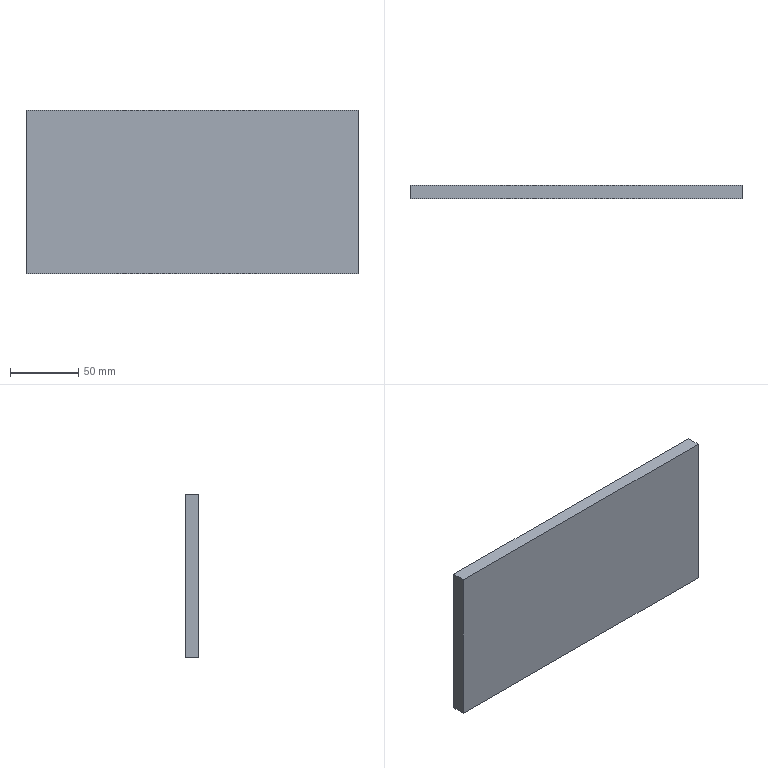Part | STEP file | 1 solid | 6 faces | box 243.554 x 10 x 120 mm | volume 292264 mm3 | plane 6
STEP:
#1=CARTESIAN_POINT('',(0.,0.,0.));
#2=DIRECTION('',(0.,0.,1.));
#3=DIRECTION('',(1.,0.,0.));
#4=AXIS2_PLACEMENT_3D('',#1,#2,#3);
#5=CARTESIAN_POINT('',(-600.,430.,-60.));
#6=VERTEX_POINT('',#5);
#7=CARTESIAN_POINT('',(-600.,430.,60.));
#8=VERTEX_POINT('',#7);
#9=CARTESIAN_POINT('',(-600.,430.,-60.));
#10=DIRECTION('',(0.,0.,1.));
#11=VECTOR('',#10,1.);
#12=LINE('',#9,#11);
#13=CARTESIAN_POINT('',(-600.,440.,-60.));
#14=DIRECTION('',(1.,0.,0.));
#15=DIRECTION('',(0.,1.,0.));
#16=AXIS2_PLACEMENT_3D('',#13,#14,#15);
#17=PLANE('',#16);
#18=CARTESIAN_POINT('',(-10.,0.));
#19=DIRECTION('',(0.,1.));
#20=VECTOR('',#19,1.);
#21=LINE('',#18,#20);
#22=(GEOMETRIC_REPRESENTATION_CONTEXT(2)PARAMETRIC_REPRESENTATION_CONTEXT()REPRESENTATION_CONTEXT('',''));
#23=DEFINITIONAL_REPRESENTATION('',(#21),#22);
#24=PCURVE('',#17,#23);
#25=CARTESIAN_POINT('',(0.,430.,0.));
#26=DIRECTION('',(0.,1.,0.));
#27=DIRECTION('',(0.,0.,1.));
#28=AXIS2_PLACEMENT_3D('',#25,#26,#27);
#29=PLANE('',#28);
#30=CARTESIAN_POINT('',(-60.,-600.));
#31=DIRECTION('',(1.,0.));
#32=VECTOR('',#31,1.);
#33=LINE('',#30,#32);
#34=(GEOMETRIC_REPRESENTATION_CONTEXT(2)PARAMETRIC_REPRESENTATION_CONTEXT()REPRESENTATION_CONTEXT('',''));
#35=DEFINITIONAL_REPRESENTATION('',(#33),#34);
#36=PCURVE('',#29,#35);
#37=SURFACE_CURVE('',#12,(#24,#36),.PCURVE_S1.);
#38=EDGE_CURVE('',#6,#8,#37,.T.);
#39=ORIENTED_EDGE('',*,*,#38,.T.);
#40=CARTESIAN_POINT('',(-600.,440.,60.));
#41=VERTEX_POINT('',#40);
#42=CARTESIAN_POINT('',(-600.,440.,60.));
#43=DIRECTION('',(0.,-1.,0.));
#44=VECTOR('',#43,1.);
#45=LINE('',#42,#44);
#46=CARTESIAN_POINT('',(0.,120.));
#47=DIRECTION('',(-1.,0.));
#48=VECTOR('',#47,1.);
#49=LINE('',#46,#48);
#50=(GEOMETRIC_REPRESENTATION_CONTEXT(2)PARAMETRIC_REPRESENTATION_CONTEXT()REPRESENTATION_CONTEXT('',''));
#51=DEFINITIONAL_REPRESENTATION('',(#49),#50);
#52=PCURVE('',#17,#51);
#53=CARTESIAN_POINT('',(-600.,440.,60.));
#54=DIRECTION('',(0.,0.,-1.));
#55=DIRECTION('',(-1.,0.,0.));
#56=AXIS2_PLACEMENT_3D('',#53,#54,#55);
#57=PLANE('',#56);
#58=CARTESIAN_POINT('',(0.,0.));
#59=DIRECTION('',(0.,-1.));
#60=VECTOR('',#59,1.);
#61=LINE('',#58,#60);
#62=(GEOMETRIC_REPRESENTATION_CONTEXT(2)PARAMETRIC_REPRESENTATION_CONTEXT()REPRESENTATION_CONTEXT('',''));
#63=DEFINITIONAL_REPRESENTATION('',(#61),#62);
#64=PCURVE('',#57,#63);
#65=SURFACE_CURVE('',#45,(#52,#64),.PCURVE_S1.);
#66=EDGE_CURVE('',#41,#8,#65,.T.);
#67=ORIENTED_EDGE('',*,*,#66,.F.);
#68=CARTESIAN_POINT('',(-600.,440.,-60.));
#69=VERTEX_POINT('',#68);
#70=CARTESIAN_POINT('',(-600.,440.,-60.));
#71=DIRECTION('',(0.,0.,1.));
#72=VECTOR('',#71,1.);
#73=LINE('',#70,#72);
#74=CARTESIAN_POINT('',(0.,0.));
#75=DIRECTION('',(0.,1.));
#76=VECTOR('',#75,1.);
#77=LINE('',#74,#76);
#78=(GEOMETRIC_REPRESENTATION_CONTEXT(2)PARAMETRIC_REPRESENTATION_CONTEXT()REPRESENTATION_CONTEXT('',''));
#79=DEFINITIONAL_REPRESENTATION('',(#77),#78);
#80=PCURVE('',#17,#79);
#81=CARTESIAN_POINT('',(0.,440.,0.));
#82=DIRECTION('',(0.,1.,0.));
#83=DIRECTION('',(0.,0.,1.));
#84=AXIS2_PLACEMENT_3D('',#81,#82,#83);
#85=PLANE('',#84);
#86=CARTESIAN_POINT('',(-60.,-600.));
#87=DIRECTION('',(1.,0.));
#88=VECTOR('',#87,1.);
#89=LINE('',#86,#88);
#90=(GEOMETRIC_REPRESENTATION_CONTEXT(2)PARAMETRIC_REPRESENTATION_CONTEXT()REPRESENTATION_CONTEXT('',''));
#91=DEFINITIONAL_REPRESENTATION('',(#89),#90);
#92=PCURVE('',#85,#91);
#93=SURFACE_CURVE('',#73,(#80,#92),.PCURVE_S1.);
#94=EDGE_CURVE('',#69,#41,#93,.T.);
#95=ORIENTED_EDGE('',*,*,#94,.F.);
#96=CARTESIAN_POINT('',(-600.,440.,-60.));
#97=DIRECTION('',(0.,-1.,0.));
#98=VECTOR('',#97,1.);
#99=LINE('',#96,#98);
#100=CARTESIAN_POINT('',(0.,0.));
#101=DIRECTION('',(-1.,0.));
#102=VECTOR('',#101,1.);
#103=LINE('',#100,#102);
#104=(GEOMETRIC_REPRESENTATION_CONTEXT(2)PARAMETRIC_REPRESENTATION_CONTEXT()REPRESENTATION_CONTEXT('',''));
#105=DEFINITIONAL_REPRESENTATION('',(#103),#104);
#106=PCURVE('',#17,#105);
#107=CARTESIAN_POINT('',(-600.,440.,-60.));
#108=DIRECTION('',(0.,0.,1.));
#109=DIRECTION('',(1.,0.,0.));
#110=AXIS2_PLACEMENT_3D('',#107,#108,#109);
#111=PLANE('',#110);
#112=CARTESIAN_POINT('',(0.,0.));
#113=DIRECTION('',(0.,-1.));
#114=VECTOR('',#113,1.);
#115=LINE('',#112,#114);
#116=(GEOMETRIC_REPRESENTATION_CONTEXT(2)PARAMETRIC_REPRESENTATION_CONTEXT()REPRESENTATION_CONTEXT('',''));
#117=DEFINITIONAL_REPRESENTATION('',(#115),#116);
#118=PCURVE('',#111,#117);
#119=SURFACE_CURVE('',#99,(#106,#118),.PCURVE_S1.);
#120=EDGE_CURVE('',#69,#6,#119,.T.);
#121=ORIENTED_EDGE('',*,*,#120,.T.);
#122=EDGE_LOOP('',(#39,#67,#95,#121));
#123=FACE_BOUND('',#122,.T.);
#124=ADVANCED_FACE('',(#123),#17,.F.);
#125=CARTESIAN_POINT('',(-356.446,430.,60.));
#126=VERTEX_POINT('',#125);
#127=CARTESIAN_POINT('',(-600.,430.,60.));
#128=DIRECTION('',(1.,0.,0.));
#129=VECTOR('',#128,1.);
#130=LINE('',#127,#129);
#131=CARTESIAN_POINT('',(0.,-10.));
#132=DIRECTION('',(-1.,0.));
#133=VECTOR('',#132,1.);
#134=LINE('',#131,#133);
#135=(GEOMETRIC_REPRESENTATION_CONTEXT(2)PARAMETRIC_REPRESENTATION_CONTEXT()REPRESENTATION_CONTEXT('',''));
#136=DEFINITIONAL_REPRESENTATION('',(#134),#135);
#137=PCURVE('',#57,#136);
#138=CARTESIAN_POINT('',(60.,-600.));
#139=DIRECTION('',(0.,1.));
#140=VECTOR('',#139,1.);
#141=LINE('',#138,#140);
#142=(GEOMETRIC_REPRESENTATION_CONTEXT(2)PARAMETRIC_REPRESENTATION_CONTEXT()REPRESENTATION_CONTEXT('',''));
#143=DEFINITIONAL_REPRESENTATION('',(#141),#142);
#144=PCURVE('',#29,#143);
#145=SURFACE_CURVE('',#130,(#137,#144),.PCURVE_S1.);
#146=EDGE_CURVE('',#8,#126,#145,.T.);
#147=ORIENTED_EDGE('',*,*,#146,.T.);
#148=CARTESIAN_POINT('',(-356.446,440.,60.));
#149=VERTEX_POINT('',#148);
#150=CARTESIAN_POINT('',(-356.446,440.,60.));
#151=DIRECTION('',(0.,-1.,0.));
#152=VECTOR('',#151,1.);
#153=LINE('',#150,#152);
#154=CARTESIAN_POINT('',(-243.554,0.));
#155=DIRECTION('',(0.,-1.));
#156=VECTOR('',#155,1.);
#157=LINE('',#154,#156);
#158=(GEOMETRIC_REPRESENTATION_CONTEXT(2)PARAMETRIC_REPRESENTATION_CONTEXT()REPRESENTATION_CONTEXT('',''));
#159=DEFINITIONAL_REPRESENTATION('',(#157),#158);
#160=PCURVE('',#57,#159);
#161=CARTESIAN_POINT('',(-356.446,440.,-60.));
#162=DIRECTION('',(-1.,0.,0.));
#163=DIRECTION('',(0.,-1.,0.));
#164=AXIS2_PLACEMENT_3D('',#161,#162,#163);
#165=PLANE('',#164);
#166=CARTESIAN_POINT('',(0.,120.));
#167=DIRECTION('',(1.,0.));
#168=VECTOR('',#167,1.);
#169=LINE('',#166,#168);
#170=(GEOMETRIC_REPRESENTATION_CONTEXT(2)PARAMETRIC_REPRESENTATION_CONTEXT()REPRESENTATION_CONTEXT('',''));
#171=DEFINITIONAL_REPRESENTATION('',(#169),#170);
#172=PCURVE('',#165,#171);
#173=SURFACE_CURVE('',#153,(#160,#172),.PCURVE_S1.);
#174=EDGE_CURVE('',#149,#126,#173,.T.);
#175=ORIENTED_EDGE('',*,*,#174,.F.);
#176=CARTESIAN_POINT('',(-600.,440.,60.));
#177=DIRECTION('',(1.,0.,0.));
#178=VECTOR('',#177,1.);
#179=LINE('',#176,#178);
#180=CARTESIAN_POINT('',(0.,0.));
#181=DIRECTION('',(-1.,0.));
#182=VECTOR('',#181,1.);
#183=LINE('',#180,#182);
#184=(GEOMETRIC_REPRESENTATION_CONTEXT(2)PARAMETRIC_REPRESENTATION_CONTEXT()REPRESENTATION_CONTEXT('',''));
#185=DEFINITIONAL_REPRESENTATION('',(#183),#184);
#186=PCURVE('',#57,#185);
#187=CARTESIAN_POINT('',(60.,-600.));
#188=DIRECTION('',(0.,1.));
#189=VECTOR('',#188,1.);
#190=LINE('',#187,#189);
#191=(GEOMETRIC_REPRESENTATION_CONTEXT(2)PARAMETRIC_REPRESENTATION_CONTEXT()REPRESENTATION_CONTEXT('',''));
#192=DEFINITIONAL_REPRESENTATION('',(#190),#191);
#193=PCURVE('',#85,#192);
#194=SURFACE_CURVE('',#179,(#186,#193),.PCURVE_S1.);
#195=EDGE_CURVE('',#41,#149,#194,.T.);
#196=ORIENTED_EDGE('',*,*,#195,.F.);
#197=ORIENTED_EDGE('',*,*,#66,.T.);
#198=EDGE_LOOP('',(#147,#175,#196,#197));
#199=FACE_BOUND('',#198,.T.);
#200=ADVANCED_FACE('',(#199),#57,.F.);
#201=CARTESIAN_POINT('',(-356.446,430.,-60.));
#202=VERTEX_POINT('',#201);
#203=CARTESIAN_POINT('',(-356.446,430.,-60.));
#204=DIRECTION('',(0.,0.,-1.));
#205=VECTOR('',#204,1.);
#206=LINE('',#203,#205);
#207=CARTESIAN_POINT('',(10.,0.));
#208=DIRECTION('',(0.,-1.));
#209=VECTOR('',#208,1.);
#210=LINE('',#207,#209);
#211=(GEOMETRIC_REPRESENTATION_CONTEXT(2)PARAMETRIC_REPRESENTATION_CONTEXT()REPRESENTATION_CONTEXT('',''));
#212=DEFINITIONAL_REPRESENTATION('',(#210),#211);
#213=PCURVE('',#165,#212);
#214=CARTESIAN_POINT('',(-60.,-356.446));
#215=DIRECTION('',(-1.,0.));
#216=VECTOR('',#215,1.);
#217=LINE('',#214,#216);
#218=(GEOMETRIC_REPRESENTATION_CONTEXT(2)PARAMETRIC_REPRESENTATION_CONTEXT()REPRESENTATION_CONTEXT('',''));
#219=DEFINITIONAL_REPRESENTATION('',(#217),#218);
#220=PCURVE('',#29,#219);
#221=SURFACE_CURVE('',#206,(#213,#220),.PCURVE_S1.);
#222=EDGE_CURVE('',#126,#202,#221,.T.);
#223=ORIENTED_EDGE('',*,*,#222,.T.);
#224=CARTESIAN_POINT('',(-356.446,440.,-60.));
#225=VERTEX_POINT('',#224);
#226=CARTESIAN_POINT('',(-356.446,440.,-60.));
#227=DIRECTION('',(0.,-1.,0.));
#228=VECTOR('',#227,1.);
#229=LINE('',#226,#228);
#230=CARTESIAN_POINT('',(0.,0.));
#231=DIRECTION('',(1.,0.));
#232=VECTOR('',#231,1.);
#233=LINE('',#230,#232);
#234=(GEOMETRIC_REPRESENTATION_CONTEXT(2)PARAMETRIC_REPRESENTATION_CONTEXT()REPRESENTATION_CONTEXT('',''));
#235=DEFINITIONAL_REPRESENTATION('',(#233),#234);
#236=PCURVE('',#165,#235);
#237=CARTESIAN_POINT('',(243.554,0.));
#238=DIRECTION('',(0.,-1.));
#239=VECTOR('',#238,1.);
#240=LINE('',#237,#239);
#241=(GEOMETRIC_REPRESENTATION_CONTEXT(2)PARAMETRIC_REPRESENTATION_CONTEXT()REPRESENTATION_CONTEXT('',''));
#242=DEFINITIONAL_REPRESENTATION('',(#240),#241);
#243=PCURVE('',#111,#242);
#244=SURFACE_CURVE('',#229,(#236,#243),.PCURVE_S1.);
#245=EDGE_CURVE('',#225,#202,#244,.T.);
#246=ORIENTED_EDGE('',*,*,#245,.F.);
#247=CARTESIAN_POINT('',(-356.446,440.,-60.));
#248=DIRECTION('',(0.,0.,-1.));
#249=VECTOR('',#248,1.);
#250=LINE('',#247,#249);
#251=CARTESIAN_POINT('',(0.,0.));
#252=DIRECTION('',(0.,-1.));
#253=VECTOR('',#252,1.);
#254=LINE('',#251,#253);
#255=(GEOMETRIC_REPRESENTATION_CONTEXT(2)PARAMETRIC_REPRESENTATION_CONTEXT()REPRESENTATION_CONTEXT('',''));
#256=DEFINITIONAL_REPRESENTATION('',(#254),#255);
#257=PCURVE('',#165,#256);
#258=CARTESIAN_POINT('',(-60.,-356.446));
#259=DIRECTION('',(-1.,0.));
#260=VECTOR('',#259,1.);
#261=LINE('',#258,#260);
#262=(GEOMETRIC_REPRESENTATION_CONTEXT(2)PARAMETRIC_REPRESENTATION_CONTEXT()REPRESENTATION_CONTEXT('',''));
#263=DEFINITIONAL_REPRESENTATION('',(#261),#262);
#264=PCURVE('',#85,#263);
#265=SURFACE_CURVE('',#250,(#257,#264),.PCURVE_S1.);
#266=EDGE_CURVE('',#149,#225,#265,.T.);
#267=ORIENTED_EDGE('',*,*,#266,.F.);
#268=ORIENTED_EDGE('',*,*,#174,.T.);
#269=EDGE_LOOP('',(#223,#246,#267,#268));
#270=FACE_BOUND('',#269,.T.);
#271=ADVANCED_FACE('',(#270),#165,.F.);
#272=CARTESIAN_POINT('',(-600.,430.,-60.));
#273=DIRECTION('',(-1.,0.,0.));
#274=VECTOR('',#273,1.);
#275=LINE('',#272,#274);
#276=CARTESIAN_POINT('',(0.,-10.));
#277=DIRECTION('',(-1.,0.));
#278=VECTOR('',#277,1.);
#279=LINE('',#276,#278);
#280=(GEOMETRIC_REPRESENTATION_CONTEXT(2)PARAMETRIC_REPRESENTATION_CONTEXT()REPRESENTATION_CONTEXT('',''));
#281=DEFINITIONAL_REPRESENTATION('',(#279),#280);
#282=PCURVE('',#111,#281);
#283=CARTESIAN_POINT('',(-60.,-600.));
#284=DIRECTION('',(0.,-1.));
#285=VECTOR('',#284,1.);
#286=LINE('',#283,#285);
#287=(GEOMETRIC_REPRESENTATION_CONTEXT(2)PARAMETRIC_REPRESENTATION_CONTEXT()REPRESENTATION_CONTEXT('',''));
#288=DEFINITIONAL_REPRESENTATION('',(#286),#287);
#289=PCURVE('',#29,#288);
#290=SURFACE_CURVE('',#275,(#282,#289),.PCURVE_S1.);
#291=EDGE_CURVE('',#202,#6,#290,.T.);
#292=ORIENTED_EDGE('',*,*,#291,.T.);
#293=ORIENTED_EDGE('',*,*,#120,.F.);
#294=CARTESIAN_POINT('',(-600.,440.,-60.));
#295=DIRECTION('',(-1.,0.,0.));
#296=VECTOR('',#295,1.);
#297=LINE('',#294,#296);
#298=CARTESIAN_POINT('',(0.,0.));
#299=DIRECTION('',(-1.,0.));
#300=VECTOR('',#299,1.);
#301=LINE('',#298,#300);
#302=(GEOMETRIC_REPRESENTATION_CONTEXT(2)PARAMETRIC_REPRESENTATION_CONTEXT()REPRESENTATION_CONTEXT('',''));
#303=DEFINITIONAL_REPRESENTATION('',(#301),#302);
#304=PCURVE('',#111,#303);
#305=CARTESIAN_POINT('',(-60.,-600.));
#306=DIRECTION('',(0.,-1.));
#307=VECTOR('',#306,1.);
#308=LINE('',#305,#307);
#309=(GEOMETRIC_REPRESENTATION_CONTEXT(2)PARAMETRIC_REPRESENTATION_CONTEXT()REPRESENTATION_CONTEXT('',''));
#310=DEFINITIONAL_REPRESENTATION('',(#308),#309);
#311=PCURVE('',#85,#310);
#312=SURFACE_CURVE('',#297,(#304,#311),.PCURVE_S1.);
#313=EDGE_CURVE('',#225,#69,#312,.T.);
#314=ORIENTED_EDGE('',*,*,#313,.F.);
#315=ORIENTED_EDGE('',*,*,#245,.T.);
#316=EDGE_LOOP('',(#292,#293,#314,#315));
#317=FACE_BOUND('',#316,.T.);
#318=ADVANCED_FACE('',(#317),#111,.F.);
#319=ORIENTED_EDGE('',*,*,#94,.T.);
#320=ORIENTED_EDGE('',*,*,#195,.T.);
#321=ORIENTED_EDGE('',*,*,#266,.T.);
#322=ORIENTED_EDGE('',*,*,#313,.T.);
#323=EDGE_LOOP('',(#319,#320,#321,#322));
#324=FACE_BOUND('',#323,.T.);
#325=ADVANCED_FACE('',(#324),#85,.T.);
#326=ORIENTED_EDGE('',*,*,#38,.F.);
#327=ORIENTED_EDGE('',*,*,#291,.F.);
#328=ORIENTED_EDGE('',*,*,#222,.F.);
#329=ORIENTED_EDGE('',*,*,#146,.F.);
#330=EDGE_LOOP('',(#326,#327,#328,#329));
#331=FACE_BOUND('',#330,.T.);
#332=ADVANCED_FACE('',(#331),#29,.F.);
#333=CLOSED_SHELL('',(#124,#200,#271,#318,#325,#332));
#334=MANIFOLD_SOLID_BREP('',#333);
#335=(LENGTH_UNIT()NAMED_UNIT(*)SI_UNIT(.MILLI.,.METRE.));
#336=UNCERTAINTY_MEASURE_WITH_UNIT(LENGTH_MEASURE(0.0000001),#335,'','');
#337=(NAMED_UNIT(*)PLANE_ANGLE_UNIT()SI_UNIT($,.RADIAN.));
#338=(NAMED_UNIT(*)SI_UNIT($,.STERADIAN.)SOLID_ANGLE_UNIT());
#339=(GEOMETRIC_REPRESENTATION_CONTEXT(3)GLOBAL_UNCERTAINTY_ASSIGNED_CONTEXT((#336))GLOBAL_UNIT_ASSIGNED_CONTEXT((#335,#337,#338))REPRESENTATION_CONTEXT('',''));
#340=ADVANCED_BREP_SHAPE_REPRESENTATION('',(#4,#334),#339);